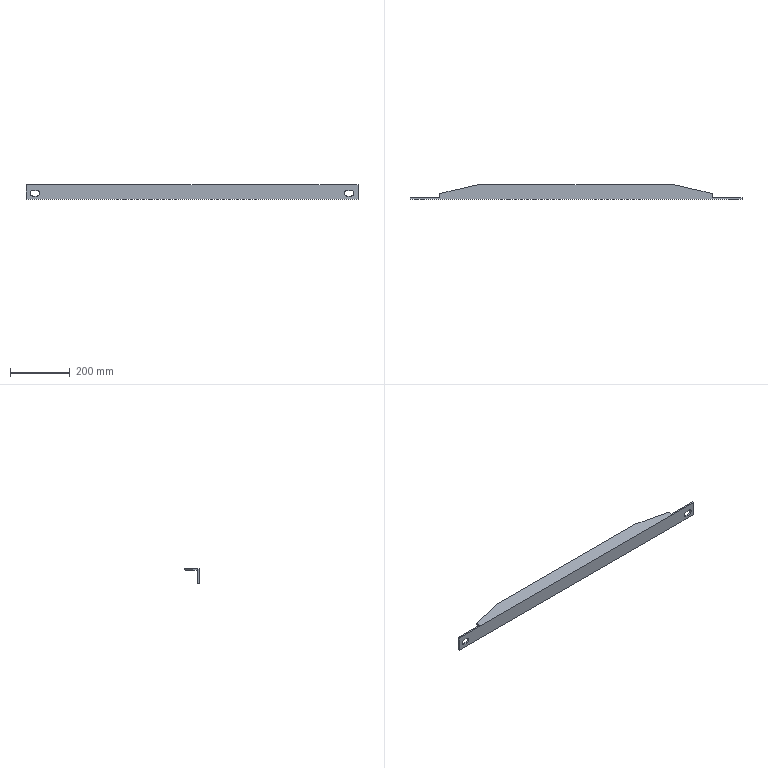Part | SolidWorks | features ICE 3, WeldMemberFeat 1, WeldmentFeature 1 | 1 solid | 23 faces | box 1113 x 50 x 50 mm | volume 463803 mm3 | plane 16 | cylinder 7 | commonest cylinder face diameters 18 x4 3.333 x2 11 x1
STEP:
#1=CARTESIAN_POINT('',(326.5,50.,-3.333));
#2=VERTEX_POINT('',#1);
#3=CARTESIAN_POINT('',(-326.5,50.,-3.333));
#4=VERTEX_POINT('',#3);
#5=CARTESIAN_POINT('',(556.5,50.,-3.333));
#6=DIRECTION('',(-1.,0.,0.));
#7=VECTOR('',#6,1000.);
#8=LINE('',#5,#7);
#9=EDGE_CURVE('',#2,#4,#8,.T.);
#10=ORIENTED_EDGE('',*,*,#9,.T.);
#11=CARTESIAN_POINT('',(-326.5,50.,0.));
#12=VERTEX_POINT('',#11);
#13=CARTESIAN_POINT('',(-326.5,50.,0.));
#14=DIRECTION('',(0.,0.,-1.));
#15=VECTOR('',#14,1000.);
#16=LINE('',#13,#15);
#17=EDGE_CURVE('',#12,#4,#16,.T.);
#18=ORIENTED_EDGE('',*,*,#17,.F.);
#19=CARTESIAN_POINT('',(326.5,50.,0.));
#20=VERTEX_POINT('',#19);
#21=CARTESIAN_POINT('',(556.5,50.,0.));
#22=DIRECTION('',(-1.,0.,0.));
#23=VECTOR('',#22,1000.);
#24=LINE('',#21,#23);
#25=EDGE_CURVE('',#20,#12,#24,.T.);
#26=ORIENTED_EDGE('',*,*,#25,.F.);
#27=CARTESIAN_POINT('',(326.5,50.,0.));
#28=DIRECTION('',(0.,0.,-1.));
#29=VECTOR('',#28,1000.);
#30=LINE('',#27,#29);
#31=EDGE_CURVE('',#20,#2,#30,.T.);
#32=ORIENTED_EDGE('',*,*,#31,.T.);
#33=EDGE_LOOP('',(#10,#18,#26,#32));
#34=FACE_OUTER_BOUND('',#33,.T.);
#35=CARTESIAN_POINT('',(556.5,50.,0.));
#36=DIRECTION('',(0.,-1.,0.));
#37=DIRECTION('',(0.,0.,-1.));
#38=AXIS2_PLACEMENT_3D('',#35,#36,#37);
#39=PLANE('',#38);
#40=ADVANCED_FACE('',(#34),#39,.F.);
#41=ORIENTED_EDGE('',*,*,#25,.T.);
#42=CARTESIAN_POINT('',(-456.5,20.,0.));
#43=VERTEX_POINT('',#42);
#44=CARTESIAN_POINT('',(-456.5,20.,0.));
#45=DIRECTION('',(-0.9744,-0.2249,0.));
#46=VECTOR('',#45,1000.);
#47=LINE('',#44,#46);
#48=EDGE_CURVE('',#12,#43,#47,.T.);
#49=ORIENTED_EDGE('',*,*,#48,.T.);
#50=CARTESIAN_POINT('',(-456.5,5.,0.));
#51=VERTEX_POINT('',#50);
#52=CARTESIAN_POINT('',(-456.5,50.001,0.));
#53=DIRECTION('',(0.,-1.,0.));
#54=VECTOR('',#53,1000.);
#55=LINE('',#52,#54);
#56=EDGE_CURVE('',#43,#51,#55,.T.);
#57=ORIENTED_EDGE('',*,*,#56,.T.);
#58=CARTESIAN_POINT('',(-556.5,5.,0.));
#59=VERTEX_POINT('',#58);
#60=CARTESIAN_POINT('',(-556.5,5.,0.));
#61=DIRECTION('',(1.,0.,0.));
#62=VECTOR('',#61,1000.);
#63=LINE('',#60,#62);
#64=EDGE_CURVE('',#59,#51,#63,.T.);
#65=ORIENTED_EDGE('',*,*,#64,.F.);
#66=CARTESIAN_POINT('',(-556.5,0.,0.));
#67=VERTEX_POINT('',#66);
#68=CARTESIAN_POINT('',(-556.5,50.,0.));
#69=DIRECTION('',(0.,-1.,0.));
#70=VECTOR('',#69,1000.);
#71=LINE('',#68,#70);
#72=EDGE_CURVE('',#59,#67,#71,.T.);
#73=ORIENTED_EDGE('',*,*,#72,.T.);
#74=CARTESIAN_POINT('',(556.5,0.,0.));
#75=VERTEX_POINT('',#74);
#76=CARTESIAN_POINT('',(556.5,0.,0.));
#77=DIRECTION('',(-1.,0.,0.));
#78=VECTOR('',#77,1000.);
#79=LINE('',#76,#78);
#80=EDGE_CURVE('',#75,#67,#79,.T.);
#81=ORIENTED_EDGE('',*,*,#80,.F.);
#82=CARTESIAN_POINT('',(556.5,5.,0.));
#83=VERTEX_POINT('',#82);
#84=CARTESIAN_POINT('',(556.5,50.,0.));
#85=DIRECTION('',(0.,-1.,0.));
#86=VECTOR('',#85,1000.);
#87=LINE('',#84,#86);
#88=EDGE_CURVE('',#83,#75,#87,.T.);
#89=ORIENTED_EDGE('',*,*,#88,.F.);
#90=CARTESIAN_POINT('',(456.5,5.,0.));
#91=VERTEX_POINT('',#90);
#92=CARTESIAN_POINT('',(556.5,5.,0.));
#93=DIRECTION('',(1.,0.,0.));
#94=VECTOR('',#93,1000.);
#95=LINE('',#92,#94);
#96=EDGE_CURVE('',#91,#83,#95,.T.);
#97=ORIENTED_EDGE('',*,*,#96,.F.);
#98=CARTESIAN_POINT('',(456.5,20.,0.));
#99=VERTEX_POINT('',#98);
#100=CARTESIAN_POINT('',(456.5,50.001,0.));
#101=DIRECTION('',(0.,-1.,0.));
#102=VECTOR('',#101,1000.);
#103=LINE('',#100,#102);
#104=EDGE_CURVE('',#99,#91,#103,.T.);
#105=ORIENTED_EDGE('',*,*,#104,.F.);
#106=CARTESIAN_POINT('',(456.5,20.,0.));
#107=DIRECTION('',(-0.9744,0.2249,0.));
#108=VECTOR('',#107,1000.);
#109=LINE('',#106,#108);
#110=EDGE_CURVE('',#99,#20,#109,.T.);
#111=ORIENTED_EDGE('',*,*,#110,.T.);
#112=EDGE_LOOP('',(#41,#49,#57,#65,#73,#81,#89,#97,#105,#111));
#113=FACE_OUTER_BOUND('',#112,.T.);
#114=CARTESIAN_POINT('',(556.5,50.,0.));
#115=DIRECTION('',(0.,0.,-1.));
#116=DIRECTION('',(0.,1.,0.));
#117=AXIS2_PLACEMENT_3D('',#114,#115,#116);
#118=PLANE('',#117);
#119=ADVANCED_FACE('',(#113),#118,.F.);
#120=CARTESIAN_POINT('',(456.5,10.5,-5.));
#121=VERTEX_POINT('',#120);
#122=CARTESIAN_POINT('',(456.5,5.,-10.5));
#123=VERTEX_POINT('',#122);
#124=CARTESIAN_POINT('',(456.5,10.5,-10.5));
#125=DIRECTION('',(1.,0.,0.));
#126=DIRECTION('',(0.,0.,-1.));
#127=AXIS2_PLACEMENT_3D('',#124,#125,#126);
#128=CIRCLE('',#127,5.5);
#129=EDGE_CURVE('',#121,#123,#128,.T.);
#130=ORIENTED_EDGE('',*,*,#129,.T.);
#131=CARTESIAN_POINT('',(-456.5,5.,-10.5));
#132=VERTEX_POINT('',#131);
#133=CARTESIAN_POINT('',(556.5,5.,-10.5));
#134=DIRECTION('',(-1.,0.,0.));
#135=VECTOR('',#134,1000.);
#136=LINE('',#133,#135);
#137=EDGE_CURVE('',#123,#132,#136,.T.);
#138=ORIENTED_EDGE('',*,*,#137,.T.);
#139=CARTESIAN_POINT('',(-456.5,10.5,-5.));
#140=VERTEX_POINT('',#139);
#141=CARTESIAN_POINT('',(-456.5,10.5,-10.5));
#142=DIRECTION('',(-1.,0.,0.));
#143=DIRECTION('',(0.,0.,1.));
#144=AXIS2_PLACEMENT_3D('',#141,#142,#143);
#145=CIRCLE('',#144,5.5);
#146=EDGE_CURVE('',#132,#140,#145,.T.);
#147=ORIENTED_EDGE('',*,*,#146,.T.);
#148=CARTESIAN_POINT('',(556.5,10.5,-5.));
#149=DIRECTION('',(-1.,0.,0.));
#150=VECTOR('',#149,1000.);
#151=LINE('',#148,#150);
#152=EDGE_CURVE('',#121,#140,#151,.T.);
#153=ORIENTED_EDGE('',*,*,#152,.F.);
#154=EDGE_LOOP('',(#130,#138,#147,#153));
#155=FACE_OUTER_BOUND('',#154,.T.);
#156=CARTESIAN_POINT('',(556.5,10.5,-10.5));
#157=DIRECTION('',(-1.,0.,0.));
#158=DIRECTION('',(0.,0.,1.));
#159=AXIS2_PLACEMENT_3D('',#156,#157,#158);
#160=CYLINDRICAL_SURFACE('',#159,5.5);
#161=ADVANCED_FACE('',(#155),#160,.F.);
#162=CARTESIAN_POINT('',(-456.5,20.,-5.));
#163=VERTEX_POINT('',#162);
#164=CARTESIAN_POINT('',(-456.5,50.001,-5.));
#165=DIRECTION('',(0.,1.,0.));
#166=VECTOR('',#165,1000.);
#167=LINE('',#164,#166);
#168=EDGE_CURVE('',#140,#163,#167,.T.);
#169=ORIENTED_EDGE('',*,*,#168,.T.);
#170=CARTESIAN_POINT('',(-333.722,48.333,-5.));
#171=VERTEX_POINT('',#170);
#172=CARTESIAN_POINT('',(511.489,243.382,-5.));
#173=DIRECTION('',(0.9744,0.2249,0.));
#174=VECTOR('',#173,1000.);
#175=LINE('',#172,#174);
#176=EDGE_CURVE('',#163,#171,#175,.T.);
#177=ORIENTED_EDGE('',*,*,#176,.T.);
#178=CARTESIAN_POINT('',(333.722,48.333,-5.));
#179=VERTEX_POINT('',#178);
#180=CARTESIAN_POINT('',(556.5,48.333,-5.));
#181=DIRECTION('',(-1.,0.,0.));
#182=VECTOR('',#181,1000.);
#183=LINE('',#180,#182);
#184=EDGE_CURVE('',#179,#171,#183,.T.);
#185=ORIENTED_EDGE('',*,*,#184,.F.);
#186=CARTESIAN_POINT('',(456.5,20.,-5.));
#187=VERTEX_POINT('',#186);
#188=CARTESIAN_POINT('',(545.236,-0.4775,-5.));
#189=DIRECTION('',(0.9744,-0.2249,0.));
#190=VECTOR('',#189,1000.);
#191=LINE('',#188,#190);
#192=EDGE_CURVE('',#179,#187,#191,.T.);
#193=ORIENTED_EDGE('',*,*,#192,.T.);
#194=CARTESIAN_POINT('',(456.5,50.001,-5.));
#195=DIRECTION('',(0.,-1.,0.));
#196=VECTOR('',#195,1000.);
#197=LINE('',#194,#196);
#198=EDGE_CURVE('',#187,#121,#197,.T.);
#199=ORIENTED_EDGE('',*,*,#198,.T.);
#200=ORIENTED_EDGE('',*,*,#152,.T.);
#201=EDGE_LOOP('',(#169,#177,#185,#193,#199,#200));
#202=FACE_OUTER_BOUND('',#201,.T.);
#203=CARTESIAN_POINT('',(556.5,48.333,-5.));
#204=DIRECTION('',(0.,0.,1.));
#205=DIRECTION('',(0.,-1.,0.));
#206=AXIS2_PLACEMENT_3D('',#203,#204,#205);
#207=PLANE('',#206);
#208=ADVANCED_FACE('',(#202),#207,.F.);
#209=ORIENTED_EDGE('',*,*,#184,.T.);
#210=CARTESIAN_POINT('',(-333.722,48.333,-5.));
#211=CARTESIAN_POINT('',(-329.492,49.31,-5.));
#212=CARTESIAN_POINT('',(-326.5,50.,-4.31));
#213=CARTESIAN_POINT('',(-326.5,50.,-3.333));
#214=(BOUNDED_CURVE()B_SPLINE_CURVE(3,(#210,#211,#212,#213),.UNSPECIFIED.,.F.,.T.)B_SPLINE_CURVE_WITH_KNOTS((4,4),(1.571,3.142),.UNSPECIFIED.)CURVE()GEOMETRIC_REPRESENTATION_ITEM()RATIONAL_B_SPLINE_CURVE((1.,0.8047,0.8047,1.))REPRESENTATION_ITEM(''));
#215=EDGE_CURVE('',#171,#4,#214,.T.);
#216=ORIENTED_EDGE('',*,*,#215,.T.);
#217=ORIENTED_EDGE('',*,*,#9,.F.);
#218=CARTESIAN_POINT('',(326.5,50.,-3.333));
#219=CARTESIAN_POINT('',(326.5,50.,-4.31));
#220=CARTESIAN_POINT('',(329.492,49.31,-5.));
#221=CARTESIAN_POINT('',(333.722,48.333,-5.));
#222=(BOUNDED_CURVE()B_SPLINE_CURVE(3,(#218,#219,#220,#221),.UNSPECIFIED.,.F.,.T.)B_SPLINE_CURVE_WITH_KNOTS((4,4),(0.,1.571),.UNSPECIFIED.)CURVE()GEOMETRIC_REPRESENTATION_ITEM()RATIONAL_B_SPLINE_CURVE((1.,0.8047,0.8047,1.))REPRESENTATION_ITEM(''));
#223=EDGE_CURVE('',#2,#179,#222,.T.);
#224=ORIENTED_EDGE('',*,*,#223,.T.);
#225=EDGE_LOOP('',(#209,#216,#217,#224));
#226=FACE_OUTER_BOUND('',#225,.T.);
#227=CARTESIAN_POINT('',(556.5,48.333,-3.333));
#228=DIRECTION('',(-1.,0.,0.));
#229=DIRECTION('',(0.,0.,1.));
#230=AXIS2_PLACEMENT_3D('',#227,#228,#229);
#231=CYLINDRICAL_SURFACE('',#230,1.667);
#232=ADVANCED_FACE('',(#226),#231,.T.);
#233=ORIENTED_EDGE('',*,*,#72,.F.);
#234=CARTESIAN_POINT('',(-556.5,5.,-48.333));
#235=VERTEX_POINT('',#234);
#236=CARTESIAN_POINT('',(-556.5,5.,-10.5));
#237=DIRECTION('',(0.,0.,1.));
#238=VECTOR('',#237,1000.);
#239=LINE('',#236,#238);
#240=EDGE_CURVE('',#235,#59,#239,.T.);
#241=ORIENTED_EDGE('',*,*,#240,.F.);
#242=CARTESIAN_POINT('',(-556.5,3.333,-50.));
#243=VERTEX_POINT('',#242);
#244=CARTESIAN_POINT('',(-556.5,3.333,-48.333));
#245=DIRECTION('',(1.,0.,0.));
#246=DIRECTION('',(0.,0.,-1.));
#247=AXIS2_PLACEMENT_3D('',#244,#245,#246);
#248=CIRCLE('',#247,1.667);
#249=EDGE_CURVE('',#243,#235,#248,.T.);
#250=ORIENTED_EDGE('',*,*,#249,.F.);
#251=CARTESIAN_POINT('',(-556.5,0.,-50.));
#252=VERTEX_POINT('',#251);
#253=CARTESIAN_POINT('',(-556.5,0.,-50.));
#254=DIRECTION('',(0.,1.,0.));
#255=VECTOR('',#254,1000.);
#256=LINE('',#253,#255);
#257=EDGE_CURVE('',#252,#243,#256,.T.);
#258=ORIENTED_EDGE('',*,*,#257,.F.);
#259=CARTESIAN_POINT('',(-556.5,0.,0.));
#260=DIRECTION('',(0.,0.,-1.));
#261=VECTOR('',#260,1000.);
#262=LINE('',#259,#261);
#263=EDGE_CURVE('',#67,#252,#262,.T.);
#264=ORIENTED_EDGE('',*,*,#263,.F.);
#265=EDGE_LOOP('',(#233,#241,#250,#258,#264));
#266=FACE_OUTER_BOUND('',#265,.T.);
#267=CARTESIAN_POINT('',(-556.5,48.333,-3.333));
#268=DIRECTION('',(-1.,0.,0.));
#269=DIRECTION('',(0.,0.,1.));
#270=AXIS2_PLACEMENT_3D('',#267,#268,#269);
#271=PLANE('',#270);
#272=ADVANCED_FACE('',(#266),#271,.T.);
#273=CARTESIAN_POINT('',(-534.,0.,-38.417));
#274=VERTEX_POINT('',#273);
#275=CARTESIAN_POINT('',(-519.,0.,-38.417));
#276=VERTEX_POINT('',#275);
#277=CARTESIAN_POINT('',(-534.,0.,-38.417));
#278=DIRECTION('',(1.,0.,0.));
#279=VECTOR('',#278,1000.);
#280=LINE('',#277,#279);
#281=EDGE_CURVE('',#274,#276,#280,.T.);
#282=ORIENTED_EDGE('',*,*,#281,.F.);
#283=CARTESIAN_POINT('',(-534.,0.,-20.417));
#284=VERTEX_POINT('',#283);
#285=CARTESIAN_POINT('',(-534.,0.,-29.417));
#286=DIRECTION('',(0.,-1.,0.));
#287=DIRECTION('',(0.,0.,1.));
#288=AXIS2_PLACEMENT_3D('',#285,#286,#287);
#289=CIRCLE('',#288,9.);
#290=EDGE_CURVE('',#284,#274,#289,.T.);
#291=ORIENTED_EDGE('',*,*,#290,.F.);
#292=CARTESIAN_POINT('',(-519.,0.,-20.417));
#293=VERTEX_POINT('',#292);
#294=CARTESIAN_POINT('',(-534.,0.,-20.417));
#295=DIRECTION('',(-1.,0.,0.));
#296=VECTOR('',#295,1000.);
#297=LINE('',#294,#296);
#298=EDGE_CURVE('',#293,#284,#297,.T.);
#299=ORIENTED_EDGE('',*,*,#298,.F.);
#300=CARTESIAN_POINT('',(-519.,0.,-29.417));
#301=DIRECTION('',(0.,-1.,0.));
#302=DIRECTION('',(0.,0.,1.));
#303=AXIS2_PLACEMENT_3D('',#300,#301,#302);
#304=CIRCLE('',#303,9.);
#305=EDGE_CURVE('',#276,#293,#304,.T.);
#306=ORIENTED_EDGE('',*,*,#305,.F.);
#307=EDGE_LOOP('',(#282,#291,#299,#306));
#308=FACE_BOUND('',#307,.T.);
#309=CARTESIAN_POINT('',(534.,0.,-20.417));
#310=VERTEX_POINT('',#309);
#311=CARTESIAN_POINT('',(519.,0.,-20.417));
#312=VERTEX_POINT('',#311);
#313=CARTESIAN_POINT('',(534.,0.,-20.417));
#314=DIRECTION('',(-1.,0.,0.));
#315=VECTOR('',#314,1000.);
#316=LINE('',#313,#315);
#317=EDGE_CURVE('',#310,#312,#316,.T.);
#318=ORIENTED_EDGE('',*,*,#317,.F.);
#319=CARTESIAN_POINT('',(534.,0.,-38.417));
#320=VERTEX_POINT('',#319);
#321=CARTESIAN_POINT('',(534.,0.,-29.417));
#322=DIRECTION('',(0.,-1.,0.));
#323=DIRECTION('',(0.,0.,1.));
#324=AXIS2_PLACEMENT_3D('',#321,#322,#323);
#325=CIRCLE('',#324,9.);
#326=EDGE_CURVE('',#320,#310,#325,.T.);
#327=ORIENTED_EDGE('',*,*,#326,.F.);
#328=CARTESIAN_POINT('',(519.,0.,-38.417));
#329=VERTEX_POINT('',#328);
#330=CARTESIAN_POINT('',(534.,0.,-38.417));
#331=DIRECTION('',(1.,0.,0.));
#332=VECTOR('',#331,1000.);
#333=LINE('',#330,#332);
#334=EDGE_CURVE('',#329,#320,#333,.T.);
#335=ORIENTED_EDGE('',*,*,#334,.F.);
#336=CARTESIAN_POINT('',(519.,0.,-29.417));
#337=DIRECTION('',(0.,-1.,0.));
#338=DIRECTION('',(0.,0.,1.));
#339=AXIS2_PLACEMENT_3D('',#336,#337,#338);
#340=CIRCLE('',#339,9.);
#341=EDGE_CURVE('',#312,#329,#340,.T.);
#342=ORIENTED_EDGE('',*,*,#341,.F.);
#343=EDGE_LOOP('',(#318,#327,#335,#342));
#344=FACE_BOUND('',#343,.T.);
#345=ORIENTED_EDGE('',*,*,#263,.T.);
#346=CARTESIAN_POINT('',(556.5,0.,-50.));
#347=VERTEX_POINT('',#346);
#348=CARTESIAN_POINT('',(556.5,0.,-50.));
#349=DIRECTION('',(-1.,0.,0.));
#350=VECTOR('',#349,1000.);
#351=LINE('',#348,#350);
#352=EDGE_CURVE('',#347,#252,#351,.T.);
#353=ORIENTED_EDGE('',*,*,#352,.F.);
#354=CARTESIAN_POINT('',(556.5,0.,0.));
#355=DIRECTION('',(0.,0.,-1.));
#356=VECTOR('',#355,1000.);
#357=LINE('',#354,#356);
#358=EDGE_CURVE('',#75,#347,#357,.T.);
#359=ORIENTED_EDGE('',*,*,#358,.F.);
#360=ORIENTED_EDGE('',*,*,#80,.T.);
#361=EDGE_LOOP('',(#345,#353,#359,#360));
#362=FACE_OUTER_BOUND('',#361,.T.);
#363=CARTESIAN_POINT('',(556.5,0.,0.));
#364=DIRECTION('',(0.,1.,0.));
#365=DIRECTION('',(0.,0.,1.));
#366=AXIS2_PLACEMENT_3D('',#363,#364,#365);
#367=PLANE('',#366);
#368=ADVANCED_FACE('',(#308,#344,#362),#367,.F.);
#369=ORIENTED_EDGE('',*,*,#257,.T.);
#370=CARTESIAN_POINT('',(556.5,3.333,-50.));
#371=VERTEX_POINT('',#370);
#372=CARTESIAN_POINT('',(556.5,3.333,-50.));
#373=DIRECTION('',(-1.,0.,0.));
#374=VECTOR('',#373,1000.);
#375=LINE('',#372,#374);
#376=EDGE_CURVE('',#371,#243,#375,.T.);
#377=ORIENTED_EDGE('',*,*,#376,.F.);
#378=CARTESIAN_POINT('',(556.5,0.,-50.));
#379=DIRECTION('',(0.,1.,0.));
#380=VECTOR('',#379,1000.);
#381=LINE('',#378,#380);
#382=EDGE_CURVE('',#347,#371,#381,.T.);
#383=ORIENTED_EDGE('',*,*,#382,.F.);
#384=ORIENTED_EDGE('',*,*,#352,.T.);
#385=EDGE_LOOP('',(#369,#377,#383,#384));
#386=FACE_OUTER_BOUND('',#385,.T.);
#387=CARTESIAN_POINT('',(556.5,0.,-50.));
#388=DIRECTION('',(0.,0.,1.));
#389=DIRECTION('',(1.,0.,0.));
#390=AXIS2_PLACEMENT_3D('',#387,#388,#389);
#391=PLANE('',#390);
#392=ADVANCED_FACE('',(#386),#391,.F.);
#393=ORIENTED_EDGE('',*,*,#249,.T.);
#394=CARTESIAN_POINT('',(556.5,5.,-48.333));
#395=VERTEX_POINT('',#394);
#396=CARTESIAN_POINT('',(556.5,5.,-48.333));
#397=DIRECTION('',(-1.,0.,0.));
#398=VECTOR('',#397,1000.);
#399=LINE('',#396,#398);
#400=EDGE_CURVE('',#395,#235,#399,.T.);
#401=ORIENTED_EDGE('',*,*,#400,.F.);
#402=CARTESIAN_POINT('',(556.5,3.333,-48.333));
#403=DIRECTION('',(1.,0.,0.));
#404=DIRECTION('',(0.,0.,-1.));
#405=AXIS2_PLACEMENT_3D('',#402,#403,#404);
#406=CIRCLE('',#405,1.667);
#407=EDGE_CURVE('',#371,#395,#406,.T.);
#408=ORIENTED_EDGE('',*,*,#407,.F.);
#409=ORIENTED_EDGE('',*,*,#376,.T.);
#410=EDGE_LOOP('',(#393,#401,#408,#409));
#411=FACE_OUTER_BOUND('',#410,.T.);
#412=CARTESIAN_POINT('',(556.5,3.333,-48.333));
#413=DIRECTION('',(-1.,0.,0.));
#414=DIRECTION('',(0.,0.,1.));
#415=AXIS2_PLACEMENT_3D('',#412,#413,#414);
#416=CYLINDRICAL_SURFACE('',#415,1.667);
#417=ADVANCED_FACE('',(#411),#416,.T.);
#418=CARTESIAN_POINT('',(-534.,5.,-20.417));
#419=VERTEX_POINT('',#418);
#420=CARTESIAN_POINT('',(-519.,5.,-20.417));
#421=VERTEX_POINT('',#420);
#422=CARTESIAN_POINT('',(-534.,5.,-20.417));
#423=DIRECTION('',(1.,0.,0.));
#424=VECTOR('',#423,1000.);
#425=LINE('',#422,#424);
#426=EDGE_CURVE('',#419,#421,#425,.T.);
#427=ORIENTED_EDGE('',*,*,#426,.F.);
#428=CARTESIAN_POINT('',(-534.,5.,-38.417));
#429=VERTEX_POINT('',#428);
#430=CARTESIAN_POINT('',(-534.,5.,-29.417));
#431=DIRECTION('',(0.,1.,0.));
#432=DIRECTION('',(0.,0.,1.));
#433=AXIS2_PLACEMENT_3D('',#430,#431,#432);
#434=CIRCLE('',#433,9.);
#435=EDGE_CURVE('',#429,#419,#434,.T.);
#436=ORIENTED_EDGE('',*,*,#435,.F.);
#437=CARTESIAN_POINT('',(-519.,5.,-38.417));
#438=VERTEX_POINT('',#437);
#439=CARTESIAN_POINT('',(-534.,5.,-38.417));
#440=DIRECTION('',(-1.,0.,0.));
#441=VECTOR('',#440,1000.);
#442=LINE('',#439,#441);
#443=EDGE_CURVE('',#438,#429,#442,.T.);
#444=ORIENTED_EDGE('',*,*,#443,.F.);
#445=CARTESIAN_POINT('',(-519.,5.,-29.417));
#446=DIRECTION('',(0.,1.,0.));
#447=DIRECTION('',(0.,0.,1.));
#448=AXIS2_PLACEMENT_3D('',#445,#446,#447);
#449=CIRCLE('',#448,9.);
#450=EDGE_CURVE('',#421,#438,#449,.T.);
#451=ORIENTED_EDGE('',*,*,#450,.F.);
#452=EDGE_LOOP('',(#427,#436,#444,#451));
#453=FACE_BOUND('',#452,.T.);
#454=CARTESIAN_POINT('',(534.,5.,-38.417));
#455=VERTEX_POINT('',#454);
#456=CARTESIAN_POINT('',(519.,5.,-38.417));
#457=VERTEX_POINT('',#456);
#458=CARTESIAN_POINT('',(534.,5.,-38.417));
#459=DIRECTION('',(-1.,0.,0.));
#460=VECTOR('',#459,1000.);
#461=LINE('',#458,#460);
#462=EDGE_CURVE('',#455,#457,#461,.T.);
#463=ORIENTED_EDGE('',*,*,#462,.F.);
#464=CARTESIAN_POINT('',(534.,5.,-20.417));
#465=VERTEX_POINT('',#464);
#466=CARTESIAN_POINT('',(534.,5.,-29.417));
#467=DIRECTION('',(0.,1.,0.));
#468=DIRECTION('',(0.,0.,1.));
#469=AXIS2_PLACEMENT_3D('',#466,#467,#468);
#470=CIRCLE('',#469,9.);
#471=EDGE_CURVE('',#465,#455,#470,.T.);
#472=ORIENTED_EDGE('',*,*,#471,.F.);
#473=CARTESIAN_POINT('',(519.,5.,-20.417));
#474=VERTEX_POINT('',#473);
#475=CARTESIAN_POINT('',(534.,5.,-20.417));
#476=DIRECTION('',(1.,0.,0.));
#477=VECTOR('',#476,1000.);
#478=LINE('',#475,#477);
#479=EDGE_CURVE('',#474,#465,#478,.T.);
#480=ORIENTED_EDGE('',*,*,#479,.F.);
#481=CARTESIAN_POINT('',(519.,5.,-29.417));
#482=DIRECTION('',(0.,1.,0.));
#483=DIRECTION('',(0.,0.,1.));
#484=AXIS2_PLACEMENT_3D('',#481,#482,#483);
#485=CIRCLE('',#484,9.);
#486=EDGE_CURVE('',#457,#474,#485,.T.);
#487=ORIENTED_EDGE('',*,*,#486,.F.);
#488=EDGE_LOOP('',(#463,#472,#480,#487));
#489=FACE_BOUND('',#488,.T.);
#490=ORIENTED_EDGE('',*,*,#240,.T.);
#491=ORIENTED_EDGE('',*,*,#64,.T.);
#492=CARTESIAN_POINT('',(-456.5,5.,-10.5));
#493=DIRECTION('',(0.,0.,-1.));
#494=VECTOR('',#493,1000.);
#495=LINE('',#492,#494);
#496=EDGE_CURVE('',#51,#132,#495,.T.);
#497=ORIENTED_EDGE('',*,*,#496,.T.);
#498=ORIENTED_EDGE('',*,*,#137,.F.);
#499=CARTESIAN_POINT('',(456.5,5.,-10.5));
#500=DIRECTION('',(0.,0.,1.));
#501=VECTOR('',#500,1000.);
#502=LINE('',#499,#501);
#503=EDGE_CURVE('',#123,#91,#502,.T.);
#504=ORIENTED_EDGE('',*,*,#503,.T.);
#505=ORIENTED_EDGE('',*,*,#96,.T.);
#506=CARTESIAN_POINT('',(556.5,5.,-10.5));
#507=DIRECTION('',(0.,0.,1.));
#508=VECTOR('',#507,1000.);
#509=LINE('',#506,#508);
#510=EDGE_CURVE('',#395,#83,#509,.T.);
#511=ORIENTED_EDGE('',*,*,#510,.F.);
#512=ORIENTED_EDGE('',*,*,#400,.T.);
#513=EDGE_LOOP('',(#490,#491,#497,#498,#504,#505,#511,#512));
#514=FACE_OUTER_BOUND('',#513,.T.);
#515=CARTESIAN_POINT('',(556.5,5.,-10.5));
#516=DIRECTION('',(0.,-1.,0.));
#517=DIRECTION('',(0.,0.,-1.));
#518=AXIS2_PLACEMENT_3D('',#515,#516,#517);
#519=PLANE('',#518);
#520=ADVANCED_FACE('',(#453,#489,#514),#519,.F.);
#521=ORIENTED_EDGE('',*,*,#510,.T.);
#522=ORIENTED_EDGE('',*,*,#88,.T.);
#523=ORIENTED_EDGE('',*,*,#358,.T.);
#524=ORIENTED_EDGE('',*,*,#382,.T.);
#525=ORIENTED_EDGE('',*,*,#407,.T.);
#526=EDGE_LOOP('',(#521,#522,#523,#524,#525));
#527=FACE_OUTER_BOUND('',#526,.T.);
#528=CARTESIAN_POINT('',(556.5,48.333,-3.333));
#529=DIRECTION('',(-1.,0.,0.));
#530=DIRECTION('',(0.,0.,1.));
#531=AXIS2_PLACEMENT_3D('',#528,#529,#530);
#532=PLANE('',#531);
#533=ADVANCED_FACE('',(#527),#532,.F.);
#534=ORIENTED_EDGE('',*,*,#326,.T.);
#535=CARTESIAN_POINT('',(534.,-0.001,-20.417));
#536=DIRECTION('',(0.,1.,0.));
#537=VECTOR('',#536,1000.);
#538=LINE('',#535,#537);
#539=EDGE_CURVE('',#310,#465,#538,.T.);
#540=ORIENTED_EDGE('',*,*,#539,.T.);
#541=ORIENTED_EDGE('',*,*,#471,.T.);
#542=CARTESIAN_POINT('',(534.,-0.001,-38.417));
#543=DIRECTION('',(0.,1.,0.));
#544=VECTOR('',#543,1000.);
#545=LINE('',#542,#544);
#546=EDGE_CURVE('',#320,#455,#545,.T.);
#547=ORIENTED_EDGE('',*,*,#546,.F.);
#548=EDGE_LOOP('',(#534,#540,#541,#547));
#549=FACE_OUTER_BOUND('',#548,.T.);
#550=CARTESIAN_POINT('',(534.,-0.001,-29.417));
#551=DIRECTION('',(0.,1.,0.));
#552=DIRECTION('',(0.,0.,1.));
#553=AXIS2_PLACEMENT_3D('',#550,#551,#552);
#554=CYLINDRICAL_SURFACE('',#553,9.);
#555=ADVANCED_FACE('',(#549),#554,.F.);
#556=ORIENTED_EDGE('',*,*,#317,.T.);
#557=CARTESIAN_POINT('',(519.,-0.001,-20.417));
#558=DIRECTION('',(0.,1.,0.));
#559=VECTOR('',#558,1000.);
#560=LINE('',#557,#559);
#561=EDGE_CURVE('',#312,#474,#560,.T.);
#562=ORIENTED_EDGE('',*,*,#561,.T.);
#563=ORIENTED_EDGE('',*,*,#479,.T.);
#564=ORIENTED_EDGE('',*,*,#539,.F.);
#565=EDGE_LOOP('',(#556,#562,#563,#564));
#566=FACE_OUTER_BOUND('',#565,.T.);
#567=CARTESIAN_POINT('',(534.,-0.001,-20.417));
#568=DIRECTION('',(0.,0.,1.));
#569=DIRECTION('',(0.,-1.,0.));
#570=AXIS2_PLACEMENT_3D('',#567,#568,#569);
#571=PLANE('',#570);
#572=ADVANCED_FACE('',(#566),#571,.F.);
#573=ORIENTED_EDGE('',*,*,#341,.T.);
#574=CARTESIAN_POINT('',(519.,-0.001,-38.417));
#575=DIRECTION('',(0.,1.,0.));
#576=VECTOR('',#575,1000.);
#577=LINE('',#574,#576);
#578=EDGE_CURVE('',#329,#457,#577,.T.);
#579=ORIENTED_EDGE('',*,*,#578,.T.);
#580=ORIENTED_EDGE('',*,*,#486,.T.);
#581=ORIENTED_EDGE('',*,*,#561,.F.);
#582=EDGE_LOOP('',(#573,#579,#580,#581));
#583=FACE_OUTER_BOUND('',#582,.T.);
#584=CARTESIAN_POINT('',(519.,-0.001,-29.417));
#585=DIRECTION('',(0.,1.,0.));
#586=DIRECTION('',(0.,0.,1.));
#587=AXIS2_PLACEMENT_3D('',#584,#585,#586);
#588=CYLINDRICAL_SURFACE('',#587,9.);
#589=ADVANCED_FACE('',(#583),#588,.F.);
#590=ORIENTED_EDGE('',*,*,#334,.T.);
#591=ORIENTED_EDGE('',*,*,#546,.T.);
#592=ORIENTED_EDGE('',*,*,#462,.T.);
#593=ORIENTED_EDGE('',*,*,#578,.F.);
#594=EDGE_LOOP('',(#590,#591,#592,#593));
#595=FACE_OUTER_BOUND('',#594,.T.);
#596=CARTESIAN_POINT('',(534.,-0.001,-38.417));
#597=DIRECTION('',(0.,0.,-1.));
#598=DIRECTION('',(0.,1.,0.));
#599=AXIS2_PLACEMENT_3D('',#596,#597,#598);
#600=PLANE('',#599);
#601=ADVANCED_FACE('',(#595),#600,.F.);
#602=ORIENTED_EDGE('',*,*,#290,.T.);
#603=CARTESIAN_POINT('',(-534.,-0.001,-38.417));
#604=DIRECTION('',(0.,1.,0.));
#605=VECTOR('',#604,1000.);
#606=LINE('',#603,#605);
#607=EDGE_CURVE('',#274,#429,#606,.T.);
#608=ORIENTED_EDGE('',*,*,#607,.T.);
#609=ORIENTED_EDGE('',*,*,#435,.T.);
#610=CARTESIAN_POINT('',(-534.,-0.001,-20.417));
#611=DIRECTION('',(0.,1.,0.));
#612=VECTOR('',#611,1000.);
#613=LINE('',#610,#612);
#614=EDGE_CURVE('',#284,#419,#613,.T.);
#615=ORIENTED_EDGE('',*,*,#614,.F.);
#616=EDGE_LOOP('',(#602,#608,#609,#615));
#617=FACE_OUTER_BOUND('',#616,.T.);
#618=CARTESIAN_POINT('',(-534.,-0.001,-29.417));
#619=DIRECTION('',(0.,1.,0.));
#620=DIRECTION('',(0.,0.,1.));
#621=AXIS2_PLACEMENT_3D('',#618,#619,#620);
#622=CYLINDRICAL_SURFACE('',#621,9.);
#623=ADVANCED_FACE('',(#617),#622,.F.);
#624=ORIENTED_EDGE('',*,*,#281,.T.);
#625=CARTESIAN_POINT('',(-519.,-0.001,-38.417));
#626=DIRECTION('',(0.,1.,0.));
#627=VECTOR('',#626,1000.);
#628=LINE('',#625,#627);
#629=EDGE_CURVE('',#276,#438,#628,.T.);
#630=ORIENTED_EDGE('',*,*,#629,.T.);
#631=ORIENTED_EDGE('',*,*,#443,.T.);
#632=ORIENTED_EDGE('',*,*,#607,.F.);
#633=EDGE_LOOP('',(#624,#630,#631,#632));
#634=FACE_OUTER_BOUND('',#633,.T.);
#635=CARTESIAN_POINT('',(-534.,-0.001,-38.417));
#636=DIRECTION('',(0.,0.,-1.));
#637=DIRECTION('',(-1.,0.,0.));
#638=AXIS2_PLACEMENT_3D('',#635,#636,#637);
#639=PLANE('',#638);
#640=ADVANCED_FACE('',(#634),#639,.F.);
#641=ORIENTED_EDGE('',*,*,#305,.T.);
#642=CARTESIAN_POINT('',(-519.,-0.001,-20.417));
#643=DIRECTION('',(0.,1.,0.));
#644=VECTOR('',#643,1000.);
#645=LINE('',#642,#644);
#646=EDGE_CURVE('',#293,#421,#645,.T.);
#647=ORIENTED_EDGE('',*,*,#646,.T.);
#648=ORIENTED_EDGE('',*,*,#450,.T.);
#649=ORIENTED_EDGE('',*,*,#629,.F.);
#650=EDGE_LOOP('',(#641,#647,#648,#649));
#651=FACE_OUTER_BOUND('',#650,.T.);
#652=CARTESIAN_POINT('',(-519.,-0.001,-29.417));
#653=DIRECTION('',(0.,1.,0.));
#654=DIRECTION('',(0.,0.,1.));
#655=AXIS2_PLACEMENT_3D('',#652,#653,#654);
#656=CYLINDRICAL_SURFACE('',#655,9.);
#657=ADVANCED_FACE('',(#651),#656,.F.);
#658=ORIENTED_EDGE('',*,*,#298,.T.);
#659=ORIENTED_EDGE('',*,*,#614,.T.);
#660=ORIENTED_EDGE('',*,*,#426,.T.);
#661=ORIENTED_EDGE('',*,*,#646,.F.);
#662=EDGE_LOOP('',(#658,#659,#660,#661));
#663=FACE_OUTER_BOUND('',#662,.T.);
#664=CARTESIAN_POINT('',(-534.,-0.001,-20.417));
#665=DIRECTION('',(0.,0.,1.));
#666=DIRECTION('',(1.,0.,0.));
#667=AXIS2_PLACEMENT_3D('',#664,#665,#666);
#668=PLANE('',#667);
#669=ADVANCED_FACE('',(#663),#668,.F.);
#670=CARTESIAN_POINT('',(-456.5,20.,0.));
#671=DIRECTION('',(0.,0.,-1.));
#672=VECTOR('',#671,1000.);
#673=LINE('',#670,#672);
#674=EDGE_CURVE('',#43,#163,#673,.T.);
#675=ORIENTED_EDGE('',*,*,#674,.T.);
#676=ORIENTED_EDGE('',*,*,#168,.F.);
#677=ORIENTED_EDGE('',*,*,#146,.F.);
#678=ORIENTED_EDGE('',*,*,#496,.F.);
#679=ORIENTED_EDGE('',*,*,#56,.F.);
#680=EDGE_LOOP('',(#675,#676,#677,#678,#679));
#681=FACE_OUTER_BOUND('',#680,.T.);
#682=CARTESIAN_POINT('',(-456.5,50.001,-10.5));
#683=DIRECTION('',(-1.,0.,0.));
#684=DIRECTION('',(0.,0.,1.));
#685=AXIS2_PLACEMENT_3D('',#682,#683,#684);
#686=PLANE('',#685);
#687=ADVANCED_FACE('',(#681),#686,.T.);
#688=CARTESIAN_POINT('',(456.5,20.,0.));
#689=DIRECTION('',(0.,0.,-1.));
#690=VECTOR('',#689,1000.);
#691=LINE('',#688,#690);
#692=EDGE_CURVE('',#99,#187,#691,.T.);
#693=ORIENTED_EDGE('',*,*,#692,.F.);
#694=ORIENTED_EDGE('',*,*,#104,.T.);
#695=ORIENTED_EDGE('',*,*,#503,.F.);
#696=ORIENTED_EDGE('',*,*,#129,.F.);
#697=ORIENTED_EDGE('',*,*,#198,.F.);
#698=EDGE_LOOP('',(#693,#694,#695,#696,#697));
#699=FACE_OUTER_BOUND('',#698,.T.);
#700=CARTESIAN_POINT('',(456.5,50.001,-10.5));
#701=DIRECTION('',(1.,0.,0.));
#702=DIRECTION('',(0.,0.,-1.));
#703=AXIS2_PLACEMENT_3D('',#700,#701,#702);
#704=PLANE('',#703);
#705=ADVANCED_FACE('',(#699),#704,.T.);
#706=ORIENTED_EDGE('',*,*,#223,.F.);
#707=ORIENTED_EDGE('',*,*,#31,.F.);
#708=ORIENTED_EDGE('',*,*,#110,.F.);
#709=ORIENTED_EDGE('',*,*,#692,.T.);
#710=ORIENTED_EDGE('',*,*,#192,.F.);
#711=EDGE_LOOP('',(#706,#707,#708,#709,#710));
#712=FACE_OUTER_BOUND('',#711,.T.);
#713=CARTESIAN_POINT('',(456.5,20.,0.));
#714=DIRECTION('',(-0.2249,-0.9744,0.));
#715=DIRECTION('',(0.9744,-0.2249,0.));
#716=AXIS2_PLACEMENT_3D('',#713,#714,#715);
#717=PLANE('',#716);
#718=ADVANCED_FACE('',(#712),#717,.F.);
#719=ORIENTED_EDGE('',*,*,#674,.F.);
#720=ORIENTED_EDGE('',*,*,#48,.F.);
#721=ORIENTED_EDGE('',*,*,#17,.T.);
#722=ORIENTED_EDGE('',*,*,#215,.F.);
#723=ORIENTED_EDGE('',*,*,#176,.F.);
#724=EDGE_LOOP('',(#719,#720,#721,#722,#723));
#725=FACE_OUTER_BOUND('',#724,.T.);
#726=CARTESIAN_POINT('',(-456.5,20.,0.));
#727=DIRECTION('',(0.2249,-0.9744,0.));
#728=DIRECTION('',(0.9744,0.2249,0.));
#729=AXIS2_PLACEMENT_3D('',#726,#727,#728);
#730=PLANE('',#729);
#731=ADVANCED_FACE('',(#725),#730,.F.);
#732=CLOSED_SHELL('',(#40,#119,#161,#208,#232,#272,#368,#392,#417,#520,#533,#555,#572,#589,#601,#623,#640,#657,#669,#687,#705,#718,#731));
#733=MANIFOLD_SOLID_BREP('',#732);
#734=CARTESIAN_POINT('',(0.,0.,0.));
#735=DIRECTION('',(0.,0.,1.));
#736=DIRECTION('',(1.,0.,0.));
#737=AXIS2_PLACEMENT_3D('',#734,#735,#736);
#738=(LENGTH_UNIT()NAMED_UNIT(*)SI_UNIT(.MILLI.,.METRE.));
#739=UNCERTAINTY_MEASURE_WITH_UNIT(LENGTH_MEASURE(0.00001),#738,'','');
#740=(NAMED_UNIT(*)PLANE_ANGLE_UNIT()SI_UNIT($,.RADIAN.));
#741=(NAMED_UNIT(*)SI_UNIT($,.STERADIAN.)SOLID_ANGLE_UNIT());
#742=(GEOMETRIC_REPRESENTATION_CONTEXT(3)GLOBAL_UNCERTAINTY_ASSIGNED_CONTEXT((#739))GLOBAL_UNIT_ASSIGNED_CONTEXT((#738,#740,#741))REPRESENTATION_CONTEXT('',''));
#743=ADVANCED_BREP_SHAPE_REPRESENTATION('',(#733,#737),#742);